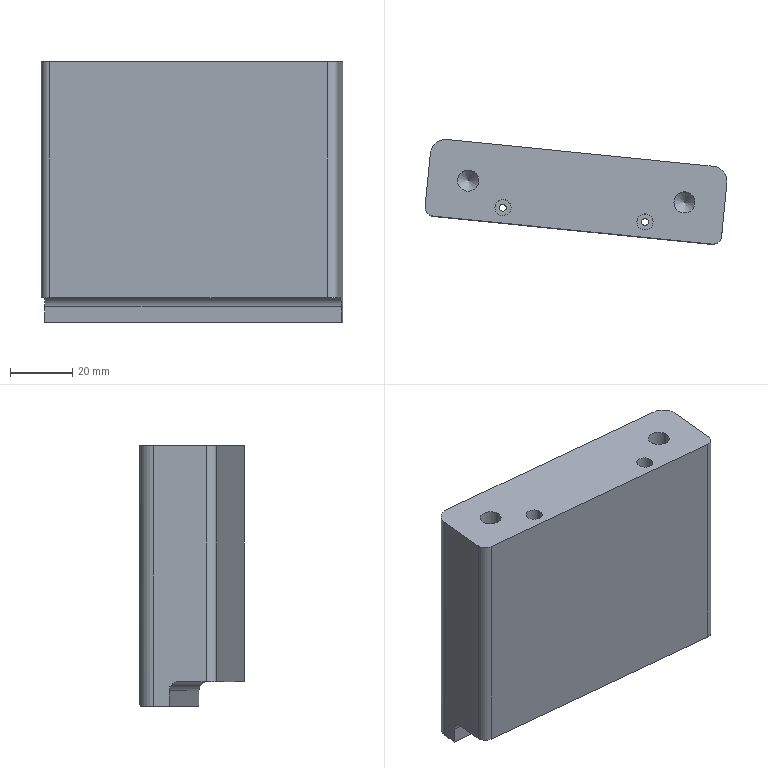Part | NX | features solid 2 | 1 solid | 26 faces | box 97.261 x 33.732 x 84 mm | volume 184630 mm3 | cylinder 13 | plane 10 | cone 3 | commonest cylinder face diameters 5.2 x3 6 x3 2.2 x2 6.8 x2 10 x2 2 x1
STEP:
#1=CARTESIAN_POINT('',(715.348,88.646,-6.));
#2=VERTEX_POINT('',#1);
#3=CARTESIAN_POINT('',(714.248,88.646,-6.));
#4=DIRECTION('',(0.,0.,1.));
#5=DIRECTION('',(1.,0.,0.));
#6=AXIS2_PLACEMENT_3D('',#3,#4,#5);
#7=CIRCLE('',#6,1.1);
#8=EDGE_CURVE('',#2,#2,#7,.F.);
#9=ORIENTED_EDGE('',*,*,#8,.F.);
#10=EDGE_LOOP('',(#9));
#11=FACE_BOUND('',#10,.T.);
#12=CARTESIAN_POINT('',(669.58,93.255,-6.));
#13=VERTEX_POINT('',#12);
#14=CARTESIAN_POINT('',(668.48,93.255,-6.));
#15=DIRECTION('',(0.,0.,1.));
#16=DIRECTION('',(1.,0.,0.));
#17=AXIS2_PLACEMENT_3D('',#14,#15,#16);
#18=CIRCLE('',#17,1.1);
#19=EDGE_CURVE('',#13,#13,#18,.F.);
#20=ORIENTED_EDGE('',*,*,#19,.F.);
#21=EDGE_LOOP('',(#20));
#22=FACE_BOUND('',#21,.T.);
#23=CARTESIAN_POINT('',(644.307,102.725,-6.));
#24=VERTEX_POINT('',#23);
#25=CARTESIAN_POINT('',(690.412,98.082,-6.));
#26=VERTEX_POINT('',#25);
#27=CARTESIAN_POINT('',(753.046,91.775,-6.));
#28=DIRECTION('',(0.995,-0.1002,0.));
#29=VECTOR('',#28,1000.);
#30=LINE('',#27,#29);
#31=EDGE_CURVE('',#24,#26,#30,.T.);
#32=ORIENTED_EDGE('',*,*,#31,.T.);
#33=CARTESIAN_POINT('',(693.718,97.749,-6.));
#34=VERTEX_POINT('',#33);
#35=CARTESIAN_POINT('',(691.865,95.926,-6.));
#36=DIRECTION('',(0.,0.,1.));
#37=DIRECTION('',(1.,0.,0.));
#38=AXIS2_PLACEMENT_3D('',#35,#36,#37);
#39=CIRCLE('',#38,2.6);
#40=EDGE_CURVE('',#26,#34,#39,.T.);
#41=ORIENTED_EDGE('',*,*,#40,.T.);
#42=CARTESIAN_POINT('',(739.824,93.106,-6.));
#43=VERTEX_POINT('',#42);
#44=CARTESIAN_POINT('',(753.046,91.775,-6.));
#45=DIRECTION('',(0.995,-0.1002,0.));
#46=VECTOR('',#45,1000.);
#47=LINE('',#44,#46);
#48=EDGE_CURVE('',#34,#43,#47,.T.);
#49=ORIENTED_EDGE('',*,*,#48,.T.);
#50=CARTESIAN_POINT('',(738.922,84.151,-6.));
#51=VERTEX_POINT('',#50);
#52=CARTESIAN_POINT('',(721.778,-86.088,-6.));
#53=DIRECTION('',(0.1002,0.995,0.));
#54=VECTOR('',#53,1000.);
#55=LINE('',#52,#54);
#56=EDGE_CURVE('',#43,#51,#55,.F.);
#57=ORIENTED_EDGE('',*,*,#56,.T.);
#58=CARTESIAN_POINT('',(735.637,81.467,-6.));
#59=VERTEX_POINT('',#58);
#60=CARTESIAN_POINT('',(735.937,84.452,-6.));
#61=DIRECTION('',(0.,0.,1.));
#62=DIRECTION('',(1.,0.,0.));
#63=AXIS2_PLACEMENT_3D('',#60,#61,#62);
#64=CIRCLE('',#63,3.);
#65=EDGE_CURVE('',#51,#59,#64,.F.);
#66=ORIENTED_EDGE('',*,*,#65,.T.);
#67=CARTESIAN_POINT('',(646.089,90.485,-6.));
#68=VERTEX_POINT('',#67);
#69=CARTESIAN_POINT('',(650.069,90.084,-6.));
#70=DIRECTION('',(-0.995,0.1002,0.));
#71=VECTOR('',#70,1000.);
#72=LINE('',#69,#71);
#73=EDGE_CURVE('',#68,#59,#72,.F.);
#74=ORIENTED_EDGE('',*,*,#73,.F.);
#75=CARTESIAN_POINT('',(643.405,93.77,-6.));
#76=VERTEX_POINT('',#75);
#77=CARTESIAN_POINT('',(646.39,93.47,-6.));
#78=DIRECTION('',(0.,0.,1.));
#79=DIRECTION('',(1.,0.,0.));
#80=AXIS2_PLACEMENT_3D('',#77,#78,#79);
#81=CIRCLE('',#80,3.);
#82=EDGE_CURVE('',#68,#76,#81,.F.);
#83=ORIENTED_EDGE('',*,*,#82,.T.);
#84=CARTESIAN_POINT('',(645.108,110.685,-6.));
#85=DIRECTION('',(0.1002,0.995,0.));
#86=VECTOR('',#85,1000.);
#87=LINE('',#84,#86);
#88=EDGE_CURVE('',#24,#76,#87,.F.);
#89=ORIENTED_EDGE('',*,*,#88,.F.);
#90=EDGE_LOOP('',(#32,#41,#49,#57,#66,#74,#83,#89));
#91=FACE_BOUND('',#90,.T.);
#92=CARTESIAN_POINT('',(735.,-87.419,-6.));
#93=DIRECTION('',(0.,0.,1.));
#94=DIRECTION('',(-0.9997,-0.02352,0.));
#95=AXIS2_PLACEMENT_3D('',#92,#93,#94);
#96=PLANE('',#95);
#97=ADVANCED_FACE('',(#11,#22,#91),#96,.F.);
#98=CARTESIAN_POINT('',(730.339,94.906,70.));
#99=VERTEX_POINT('',#98);
#100=CARTESIAN_POINT('',(726.939,94.906,70.));
#101=DIRECTION('',(0.,0.,-1.));
#102=DIRECTION('',(1.,0.,0.));
#103=AXIS2_PLACEMENT_3D('',#100,#101,#102);
#104=CIRCLE('',#103,3.4);
#105=EDGE_CURVE('',#99,#99,#104,.T.);
#106=ORIENTED_EDGE('',*,*,#105,.T.);
#107=EDGE_LOOP('',(#106));
#108=FACE_BOUND('',#107,.T.);
#109=CARTESIAN_POINT('',(671.08,93.255,70.));
#110=VERTEX_POINT('',#109);
#111=CARTESIAN_POINT('',(668.48,93.255,70.));
#112=DIRECTION('',(0.,0.,1.));
#113=DIRECTION('',(1.,0.,0.));
#114=AXIS2_PLACEMENT_3D('',#111,#112,#113);
#115=CIRCLE('',#114,2.6);
#116=EDGE_CURVE('',#110,#110,#115,.T.);
#117=ORIENTED_EDGE('',*,*,#116,.F.);
#118=EDGE_LOOP('',(#117));
#119=FACE_BOUND('',#118,.T.);
#120=CARTESIAN_POINT('',(716.848,88.646,70.));
#121=VERTEX_POINT('',#120);
#122=CARTESIAN_POINT('',(714.248,88.646,70.));
#123=DIRECTION('',(0.,0.,1.));
#124=DIRECTION('',(1.,0.,0.));
#125=AXIS2_PLACEMENT_3D('',#122,#123,#124);
#126=CIRCLE('',#125,2.6);
#127=EDGE_CURVE('',#121,#121,#126,.T.);
#128=ORIENTED_EDGE('',*,*,#127,.F.);
#129=EDGE_LOOP('',(#128));
#130=FACE_BOUND('',#129,.T.);
#131=CARTESIAN_POINT('',(740.625,101.066,70.));
#132=VERTEX_POINT('',#131);
#133=CARTESIAN_POINT('',(738.922,84.151,70.));
#134=VERTEX_POINT('',#133);
#135=CARTESIAN_POINT('',(740.625,101.066,70.));
#136=DIRECTION('',(-0.1002,-0.995,0.));
#137=VECTOR('',#136,1000.);
#138=LINE('',#135,#137);
#139=EDGE_CURVE('',#132,#134,#138,.T.);
#140=ORIENTED_EDGE('',*,*,#139,.F.);
#141=CARTESIAN_POINT('',(736.152,106.542,70.));
#142=VERTEX_POINT('',#141);
#143=CARTESIAN_POINT('',(735.651,101.567,70.));
#144=DIRECTION('',(0.,0.,1.));
#145=DIRECTION('',(1.,0.,0.));
#146=AXIS2_PLACEMENT_3D('',#143,#144,#145);
#147=CIRCLE('',#146,5.);
#148=EDGE_CURVE('',#132,#142,#147,.T.);
#149=ORIENTED_EDGE('',*,*,#148,.T.);
#150=CARTESIAN_POINT('',(650.584,115.159,70.));
#151=VERTEX_POINT('',#150);
#152=CARTESIAN_POINT('',(652.574,114.958,70.));
#153=DIRECTION('',(-0.995,0.1002,0.));
#154=VECTOR('',#153,1000.);
#155=LINE('',#152,#154);
#156=EDGE_CURVE('',#142,#151,#155,.T.);
#157=ORIENTED_EDGE('',*,*,#156,.T.);
#158=CARTESIAN_POINT('',(645.108,110.685,70.));
#159=VERTEX_POINT('',#158);
#160=CARTESIAN_POINT('',(650.083,110.184,70.));
#161=DIRECTION('',(0.,0.,1.));
#162=DIRECTION('',(1.,0.,0.));
#163=AXIS2_PLACEMENT_3D('',#160,#161,#162);
#164=CIRCLE('',#163,5.);
#165=EDGE_CURVE('',#151,#159,#164,.T.);
#166=ORIENTED_EDGE('',*,*,#165,.T.);
#167=CARTESIAN_POINT('',(643.405,93.77,70.));
#168=VERTEX_POINT('',#167);
#169=CARTESIAN_POINT('',(633.24,-7.174,70.));
#170=DIRECTION('',(-0.1002,-0.995,0.));
#171=VECTOR('',#170,1000.);
#172=LINE('',#169,#171);
#173=EDGE_CURVE('',#159,#168,#172,.T.);
#174=ORIENTED_EDGE('',*,*,#173,.T.);
#175=CARTESIAN_POINT('',(646.089,90.485,70.));
#176=VERTEX_POINT('',#175);
#177=CARTESIAN_POINT('',(646.39,93.47,70.));
#178=DIRECTION('',(0.,0.,1.));
#179=DIRECTION('',(1.,0.,0.));
#180=AXIS2_PLACEMENT_3D('',#177,#178,#179);
#181=CIRCLE('',#180,3.);
#182=EDGE_CURVE('',#168,#176,#181,.T.);
#183=ORIENTED_EDGE('',*,*,#182,.T.);
#184=CARTESIAN_POINT('',(735.637,81.467,70.));
#185=VERTEX_POINT('',#184);
#186=CARTESIAN_POINT('',(650.069,90.084,70.));
#187=DIRECTION('',(-0.995,0.1002,0.));
#188=VECTOR('',#187,1000.);
#189=LINE('',#186,#188);
#190=EDGE_CURVE('',#185,#176,#189,.T.);
#191=ORIENTED_EDGE('',*,*,#190,.F.);
#192=CARTESIAN_POINT('',(735.937,84.452,70.));
#193=DIRECTION('',(0.,0.,1.));
#194=DIRECTION('',(1.,0.,0.));
#195=AXIS2_PLACEMENT_3D('',#192,#193,#194);
#196=CIRCLE('',#195,3.);
#197=EDGE_CURVE('',#185,#134,#196,.T.);
#198=ORIENTED_EDGE('',*,*,#197,.T.);
#199=EDGE_LOOP('',(#140,#149,#157,#166,#174,#183,#191,#198));
#200=FACE_BOUND('',#199,.T.);
#201=CARTESIAN_POINT('',(660.692,101.92,70.));
#202=VERTEX_POINT('',#201);
#203=CARTESIAN_POINT('',(657.292,101.92,70.));
#204=DIRECTION('',(0.,0.,-1.));
#205=DIRECTION('',(1.,0.,0.));
#206=AXIS2_PLACEMENT_3D('',#203,#204,#205);
#207=CIRCLE('',#206,3.4);
#208=EDGE_CURVE('',#202,#202,#207,.T.);
#209=ORIENTED_EDGE('',*,*,#208,.T.);
#210=EDGE_LOOP('',(#209));
#211=FACE_BOUND('',#210,.T.);
#212=CARTESIAN_POINT('',(562.,0.,70.));
#213=DIRECTION('',(0.,0.,1.));
#214=DIRECTION('',(1.,0.,0.));
#215=AXIS2_PLACEMENT_3D('',#212,#213,#214);
#216=PLANE('',#215);
#217=ADVANCED_FACE('',(#108,#119,#130,#200,#211),#216,.T.);
#218=ORIENTED_EDGE('',*,*,#173,.F.);
#219=CARTESIAN_POINT('',(645.108,110.685,-14.));
#220=VERTEX_POINT('',#219);
#221=CARTESIAN_POINT('',(645.108,110.685,-14.));
#222=DIRECTION('',(0.,0.,-1.));
#223=VECTOR('',#222,1000.);
#224=LINE('',#221,#223);
#225=EDGE_CURVE('',#159,#220,#224,.T.);
#226=ORIENTED_EDGE('',*,*,#225,.T.);
#227=CARTESIAN_POINT('',(644.607,105.71,-14.));
#228=VERTEX_POINT('',#227);
#229=CARTESIAN_POINT('',(645.108,110.685,-14.));
#230=DIRECTION('',(-0.1002,-0.995,0.));
#231=VECTOR('',#230,1000.);
#232=LINE('',#229,#231);
#233=EDGE_CURVE('',#220,#228,#232,.T.);
#234=ORIENTED_EDGE('',*,*,#233,.T.);
#235=CARTESIAN_POINT('',(644.607,105.71,-9.));
#236=VERTEX_POINT('',#235);
#237=CARTESIAN_POINT('',(644.607,105.71,-41.49));
#238=DIRECTION('',(0.,0.,-1.));
#239=VECTOR('',#238,1000.);
#240=LINE('',#237,#239);
#241=EDGE_CURVE('',#228,#236,#240,.F.);
#242=ORIENTED_EDGE('',*,*,#241,.T.);
#243=CARTESIAN_POINT('',(644.307,102.725,-9.));
#244=DIRECTION('',(-0.995,0.1002,0.));
#245=DIRECTION('',(-0.1002,-0.995,0.));
#246=AXIS2_PLACEMENT_3D('',#243,#244,#245);
#247=CIRCLE('',#246,3.);
#248=EDGE_CURVE('',#236,#24,#247,.F.);
#249=ORIENTED_EDGE('',*,*,#248,.T.);
#250=ORIENTED_EDGE('',*,*,#88,.T.);
#251=CARTESIAN_POINT('',(643.405,93.77,-41.49));
#252=DIRECTION('',(0.,0.,-1.));
#253=VECTOR('',#252,1000.);
#254=LINE('',#251,#253);
#255=EDGE_CURVE('',#76,#168,#254,.F.);
#256=ORIENTED_EDGE('',*,*,#255,.T.);
#257=EDGE_LOOP('',(#218,#226,#234,#242,#249,#250,#256));
#258=FACE_BOUND('',#257,.T.);
#259=CARTESIAN_POINT('',(645.108,110.685,-41.49));
#260=DIRECTION('',(-0.995,0.1002,0.));
#261=DIRECTION('',(-0.1002,-0.995,0.));
#262=AXIS2_PLACEMENT_3D('',#259,#260,#261);
#263=PLANE('',#262);
#264=ADVANCED_FACE('',(#258),#263,.T.);
#265=CARTESIAN_POINT('',(740.625,101.066,-14.));
#266=VERTEX_POINT('',#265);
#267=CARTESIAN_POINT('',(740.124,96.091,-14.));
#268=VERTEX_POINT('',#267);
#269=CARTESIAN_POINT('',(712.51,-178.12,-14.));
#270=DIRECTION('',(-0.1002,-0.995,0.));
#271=VECTOR('',#270,1000.);
#272=LINE('',#269,#271);
#273=EDGE_CURVE('',#266,#268,#272,.T.);
#274=ORIENTED_EDGE('',*,*,#273,.F.);
#275=CARTESIAN_POINT('',(740.625,101.066,50.));
#276=DIRECTION('',(0.,0.,1.));
#277=VECTOR('',#276,1000.);
#278=LINE('',#275,#277);
#279=EDGE_CURVE('',#266,#132,#278,.T.);
#280=ORIENTED_EDGE('',*,*,#279,.T.);
#281=ORIENTED_EDGE('',*,*,#139,.T.);
#282=CARTESIAN_POINT('',(738.922,84.151,-41.49));
#283=DIRECTION('',(0.,0.,1.));
#284=VECTOR('',#283,1000.);
#285=LINE('',#282,#284);
#286=EDGE_CURVE('',#134,#51,#285,.F.);
#287=ORIENTED_EDGE('',*,*,#286,.T.);
#288=ORIENTED_EDGE('',*,*,#56,.F.);
#289=CARTESIAN_POINT('',(740.124,96.091,-9.));
#290=VERTEX_POINT('',#289);
#291=CARTESIAN_POINT('',(739.824,93.106,-9.));
#292=DIRECTION('',(0.995,-0.1002,0.));
#293=DIRECTION('',(0.1002,0.995,0.));
#294=AXIS2_PLACEMENT_3D('',#291,#292,#293);
#295=CIRCLE('',#294,3.);
#296=EDGE_CURVE('',#43,#290,#295,.F.);
#297=ORIENTED_EDGE('',*,*,#296,.T.);
#298=CARTESIAN_POINT('',(740.124,96.091,-41.49));
#299=DIRECTION('',(0.,0.,1.));
#300=VECTOR('',#299,1000.);
#301=LINE('',#298,#300);
#302=EDGE_CURVE('',#268,#290,#301,.T.);
#303=ORIENTED_EDGE('',*,*,#302,.F.);
#304=EDGE_LOOP('',(#274,#280,#281,#287,#288,#297,#303));
#305=FACE_BOUND('',#304,.T.);
#306=CARTESIAN_POINT('',(740.625,101.066,-41.49));
#307=DIRECTION('',(0.995,-0.1002,0.));
#308=DIRECTION('',(0.1002,0.995,0.));
#309=AXIS2_PLACEMENT_3D('',#306,#307,#308);
#310=PLANE('',#309);
#311=ADVANCED_FACE('',(#305),#310,.T.);
#312=ORIENTED_EDGE('',*,*,#73,.T.);
#313=CARTESIAN_POINT('',(735.637,81.467,-41.49));
#314=DIRECTION('',(0.,0.,1.));
#315=VECTOR('',#314,1000.);
#316=LINE('',#313,#315);
#317=EDGE_CURVE('',#59,#185,#316,.T.);
#318=ORIENTED_EDGE('',*,*,#317,.T.);
#319=ORIENTED_EDGE('',*,*,#190,.T.);
#320=CARTESIAN_POINT('',(646.089,90.485,-41.49));
#321=DIRECTION('',(0.,0.,-1.));
#322=VECTOR('',#321,1000.);
#323=LINE('',#320,#322);
#324=EDGE_CURVE('',#176,#68,#323,.T.);
#325=ORIENTED_EDGE('',*,*,#324,.T.);
#326=EDGE_LOOP('',(#312,#318,#319,#325));
#327=FACE_BOUND('',#326,.T.);
#328=CARTESIAN_POINT('',(650.069,90.084,-41.49));
#329=DIRECTION('',(-0.1002,-0.995,0.));
#330=DIRECTION('',(0.995,-0.1002,0.));
#331=AXIS2_PLACEMENT_3D('',#328,#329,#330);
#332=PLANE('',#331);
#333=ADVANCED_FACE('',(#327),#332,.T.);
#334=ORIENTED_EDGE('',*,*,#65,.F.);
#335=ORIENTED_EDGE('',*,*,#286,.F.);
#336=ORIENTED_EDGE('',*,*,#197,.F.);
#337=ORIENTED_EDGE('',*,*,#317,.F.);
#338=EDGE_LOOP('',(#334,#335,#336,#337));
#339=FACE_BOUND('',#338,.T.);
#340=CARTESIAN_POINT('',(735.937,84.452,-41.49));
#341=DIRECTION('',(0.,0.,1.));
#342=DIRECTION('',(1.,0.,0.));
#343=AXIS2_PLACEMENT_3D('',#340,#341,#342);
#344=CYLINDRICAL_SURFACE('',#343,3.);
#345=ADVANCED_FACE('',(#339),#344,.T.);
#346=ORIENTED_EDGE('',*,*,#182,.F.);
#347=ORIENTED_EDGE('',*,*,#255,.F.);
#348=ORIENTED_EDGE('',*,*,#82,.F.);
#349=ORIENTED_EDGE('',*,*,#324,.F.);
#350=EDGE_LOOP('',(#346,#347,#348,#349));
#351=FACE_BOUND('',#350,.T.);
#352=CARTESIAN_POINT('',(646.39,93.47,-41.49));
#353=DIRECTION('',(0.,0.,-1.));
#354=DIRECTION('',(-1.,0.,0.));
#355=AXIS2_PLACEMENT_3D('',#352,#353,#354);
#356=CYLINDRICAL_SURFACE('',#355,3.);
#357=ADVANCED_FACE('',(#351),#356,.T.);
#358=CARTESIAN_POINT('',(736.152,106.542,-13.));
#359=VERTEX_POINT('',#358);
#360=CARTESIAN_POINT('',(736.152,106.542,-14.));
#361=DIRECTION('',(0.,0.,1.));
#362=VECTOR('',#361,1000.);
#363=LINE('',#360,#362);
#364=EDGE_CURVE('',#142,#359,#363,.F.);
#365=ORIENTED_EDGE('',*,*,#364,.T.);
#366=CARTESIAN_POINT('',(650.584,115.159,-13.));
#367=VERTEX_POINT('',#366);
#368=CARTESIAN_POINT('',(650.584,115.159,-13.));
#369=DIRECTION('',(0.995,-0.1002,0.));
#370=VECTOR('',#369,1000.);
#371=LINE('',#368,#370);
#372=EDGE_CURVE('',#359,#367,#371,.F.);
#373=ORIENTED_EDGE('',*,*,#372,.T.);
#374=CARTESIAN_POINT('',(650.584,115.159,50.));
#375=DIRECTION('',(0.,0.,-1.));
#376=VECTOR('',#375,1000.);
#377=LINE('',#374,#376);
#378=EDGE_CURVE('',#367,#151,#377,.F.);
#379=ORIENTED_EDGE('',*,*,#378,.T.);
#380=ORIENTED_EDGE('',*,*,#156,.F.);
#381=EDGE_LOOP('',(#365,#373,#379,#380));
#382=FACE_BOUND('',#381,.T.);
#383=CARTESIAN_POINT('',(652.574,114.958,-41.49));
#384=DIRECTION('',(-0.1002,-0.995,0.));
#385=DIRECTION('',(0.995,-0.1002,0.));
#386=AXIS2_PLACEMENT_3D('',#383,#384,#385);
#387=PLANE('',#386);
#388=ADVANCED_FACE('',(#382),#387,.F.);
#389=CARTESIAN_POINT('',(647.499,114.464,-14.));
#390=VERTEX_POINT('',#389);
#391=CARTESIAN_POINT('',(650.083,110.184,-14.));
#392=DIRECTION('',(0.,0.,-1.));
#393=DIRECTION('',(-1.,0.,0.));
#394=AXIS2_PLACEMENT_3D('',#391,#392,#393);
#395=CIRCLE('',#394,5.);
#396=EDGE_CURVE('',#220,#390,#395,.T.);
#397=ORIENTED_EDGE('',*,*,#396,.T.);
#398=CARTESIAN_POINT('',(739.036,105.246,-14.));
#399=VERTEX_POINT('',#398);
#400=CARTESIAN_POINT('',(736.051,105.547,-14.));
#401=DIRECTION('',(0.995,-0.1002,0.));
#402=VECTOR('',#401,1000.);
#403=LINE('',#400,#402);
#404=EDGE_CURVE('',#390,#399,#403,.T.);
#405=ORIENTED_EDGE('',*,*,#404,.T.);
#406=CARTESIAN_POINT('',(735.651,101.567,-14.));
#407=DIRECTION('',(0.,0.,-1.));
#408=DIRECTION('',(-1.,0.,0.));
#409=AXIS2_PLACEMENT_3D('',#406,#407,#408);
#410=CIRCLE('',#409,5.);
#411=EDGE_CURVE('',#399,#266,#410,.T.);
#412=ORIENTED_EDGE('',*,*,#411,.T.);
#413=ORIENTED_EDGE('',*,*,#273,.T.);
#414=CARTESIAN_POINT('',(692.366,100.901,-14.));
#415=DIRECTION('',(-0.995,0.1002,0.));
#416=VECTOR('',#415,1000.);
#417=LINE('',#414,#416);
#418=EDGE_CURVE('',#268,#228,#417,.T.);
#419=ORIENTED_EDGE('',*,*,#418,.T.);
#420=ORIENTED_EDGE('',*,*,#233,.F.);
#421=EDGE_LOOP('',(#397,#405,#412,#413,#419,#420));
#422=FACE_BOUND('',#421,.T.);
#423=CARTESIAN_POINT('',(16.212,-108.,-14.));
#424=DIRECTION('',(0.,0.,-1.));
#425=DIRECTION('',(-1.,0.,0.));
#426=AXIS2_PLACEMENT_3D('',#423,#424,#425);
#427=PLANE('',#426);
#428=ADVANCED_FACE('',(#422),#427,.T.);
#429=ORIENTED_EDGE('',*,*,#302,.T.);
#430=CARTESIAN_POINT('',(692.366,100.901,-9.));
#431=DIRECTION('',(-0.995,0.1002,0.));
#432=VECTOR('',#431,1000.);
#433=LINE('',#430,#432);
#434=EDGE_CURVE('',#290,#236,#433,.T.);
#435=ORIENTED_EDGE('',*,*,#434,.T.);
#436=ORIENTED_EDGE('',*,*,#241,.F.);
#437=ORIENTED_EDGE('',*,*,#418,.F.);
#438=EDGE_LOOP('',(#429,#435,#436,#437));
#439=FACE_BOUND('',#438,.T.);
#440=CARTESIAN_POINT('',(692.366,100.901,18.));
#441=DIRECTION('',(0.1002,0.995,0.));
#442=DIRECTION('',(-0.995,0.1002,0.));
#443=AXIS2_PLACEMENT_3D('',#440,#441,#442);
#444=PLANE('',#443);
#445=ADVANCED_FACE('',(#439),#444,.F.);
#446=ORIENTED_EDGE('',*,*,#411,.F.);
#447=CARTESIAN_POINT('',(739.036,105.246,-14.));
#448=CARTESIAN_POINT('',(738.194,106.021,-14.));
#449=CARTESIAN_POINT('',(737.177,106.438,-13.461));
#450=CARTESIAN_POINT('',(736.152,106.542,-13.));
#451=B_SPLINE_CURVE_WITH_KNOTS('',3,(#447,#448,#449,#450),.UNSPECIFIED.,.F.,.F.,(4,4),(0.,0.003386),.UNSPECIFIED.);
#452=EDGE_CURVE('',#399,#359,#451,.T.);
#453=ORIENTED_EDGE('',*,*,#452,.T.);
#454=ORIENTED_EDGE('',*,*,#364,.F.);
#455=ORIENTED_EDGE('',*,*,#148,.F.);
#456=ORIENTED_EDGE('',*,*,#279,.F.);
#457=EDGE_LOOP('',(#446,#453,#454,#455,#456));
#458=FACE_BOUND('',#457,.T.);
#459=CARTESIAN_POINT('',(735.651,101.567,-41.49));
#460=DIRECTION('',(0.,0.,-1.));
#461=DIRECTION('',(-1.,0.,0.));
#462=AXIS2_PLACEMENT_3D('',#459,#460,#461);
#463=CYLINDRICAL_SURFACE('',#462,5.);
#464=ADVANCED_FACE('',(#458),#463,.T.);
#465=ORIENTED_EDGE('',*,*,#378,.F.);
#466=CARTESIAN_POINT('',(647.499,114.464,-14.));
#467=CARTESIAN_POINT('',(648.478,115.056,-14.));
#468=CARTESIAN_POINT('',(649.559,115.262,-13.461));
#469=CARTESIAN_POINT('',(650.584,115.159,-13.));
#470=B_SPLINE_CURVE_WITH_KNOTS('',3,(#466,#467,#468,#469),.UNSPECIFIED.,.F.,.F.,(4,4),(0.,0.003386),.UNSPECIFIED.);
#471=EDGE_CURVE('',#367,#390,#470,.F.);
#472=ORIENTED_EDGE('',*,*,#471,.T.);
#473=ORIENTED_EDGE('',*,*,#396,.F.);
#474=ORIENTED_EDGE('',*,*,#225,.F.);
#475=ORIENTED_EDGE('',*,*,#165,.F.);
#476=EDGE_LOOP('',(#465,#472,#473,#474,#475));
#477=FACE_BOUND('',#476,.T.);
#478=CARTESIAN_POINT('',(650.083,110.184,-41.49));
#479=DIRECTION('',(0.,0.,1.));
#480=DIRECTION('',(1.,0.,0.));
#481=AXIS2_PLACEMENT_3D('',#478,#479,#480);
#482=CYLINDRICAL_SURFACE('',#481,5.);
#483=ADVANCED_FACE('',(#477),#482,.T.);
#484=CARTESIAN_POINT('',(690.412,98.082,-6.));
#485=CARTESIAN_POINT('',(690.916,98.421,-6.));
#486=CARTESIAN_POINT('',(692.146,98.724,-6.121));
#487=CARTESIAN_POINT('',(693.293,98.182,-6.));
#488=CARTESIAN_POINT('',(693.718,97.749,-6.));
#489=B_SPLINE_CURVE_WITH_KNOTS('',3,(#484,#485,#486,#487,#488),.UNSPECIFIED.,.F.,.F.,(4,1,4),(0.,0.001794,0.003588),.UNSPECIFIED.);
#490=EDGE_CURVE('',#26,#34,#489,.T.);
#491=ORIENTED_EDGE('',*,*,#490,.F.);
#492=ORIENTED_EDGE('',*,*,#31,.F.);
#493=ORIENTED_EDGE('',*,*,#248,.F.);
#494=ORIENTED_EDGE('',*,*,#434,.F.);
#495=ORIENTED_EDGE('',*,*,#296,.F.);
#496=ORIENTED_EDGE('',*,*,#48,.F.);
#497=EDGE_LOOP('',(#491,#492,#493,#494,#495,#496));
#498=FACE_BOUND('',#497,.T.);
#499=CARTESIAN_POINT('',(753.046,91.775,-9.));
#500=DIRECTION('',(-0.995,0.1002,0.));
#501=DIRECTION('',(-0.1002,-0.995,0.));
#502=AXIS2_PLACEMENT_3D('',#499,#500,#501);
#503=CYLINDRICAL_SURFACE('',#502,3.);
#504=ADVANCED_FACE('',(#498),#503,.F.);
#505=ORIENTED_EDGE('',*,*,#8,.T.);
#506=EDGE_LOOP('',(#505));
#507=FACE_BOUND('',#506,.T.);
#508=CARTESIAN_POINT('',(713.148,88.646,29.));
#509=VERTEX_POINT('',#508);
#510=CARTESIAN_POINT('',(714.248,88.646,29.));
#511=DIRECTION('',(0.,0.,-1.));
#512=DIRECTION('',(-1.,0.,0.));
#513=AXIS2_PLACEMENT_3D('',#510,#511,#512);
#514=CIRCLE('',#513,1.1);
#515=EDGE_CURVE('',#509,#509,#514,.T.);
#516=ORIENTED_EDGE('',*,*,#515,.F.);
#517=EDGE_LOOP('',(#516));
#518=FACE_BOUND('',#517,.T.);
#519=CARTESIAN_POINT('',(714.248,88.646,32.));
#520=DIRECTION('',(0.,0.,-1.));
#521=DIRECTION('',(1.,0.,0.));
#522=AXIS2_PLACEMENT_3D('',#519,#520,#521);
#523=CYLINDRICAL_SURFACE('',#522,1.1);
#524=ADVANCED_FACE('',(#507,#518),#523,.F.);
#525=ORIENTED_EDGE('',*,*,#515,.T.);
#526=EDGE_LOOP('',(#525));
#527=FACE_BOUND('',#526,.T.);
#528=CARTESIAN_POINT('',(716.848,88.646,29.));
#529=VERTEX_POINT('',#528);
#530=CARTESIAN_POINT('',(714.248,88.646,29.));
#531=DIRECTION('',(0.,0.,1.));
#532=DIRECTION('',(1.,0.,0.));
#533=AXIS2_PLACEMENT_3D('',#530,#531,#532);
#534=CIRCLE('',#533,2.6);
#535=EDGE_CURVE('',#529,#529,#534,.F.);
#536=ORIENTED_EDGE('',*,*,#535,.F.);
#537=EDGE_LOOP('',(#536));
#538=FACE_BOUND('',#537,.T.);
#539=CARTESIAN_POINT('',(714.248,88.646,29.));
#540=DIRECTION('',(0.,0.,-1.));
#541=DIRECTION('',(-1.,0.,0.));
#542=AXIS2_PLACEMENT_3D('',#539,#540,#541);
#543=PLANE('',#542);
#544=ADVANCED_FACE('',(#527,#538),#543,.F.);
#545=ORIENTED_EDGE('',*,*,#127,.T.);
#546=EDGE_LOOP('',(#545));
#547=FACE_BOUND('',#546,.T.);
#548=ORIENTED_EDGE('',*,*,#535,.T.);
#549=EDGE_LOOP('',(#548));
#550=FACE_BOUND('',#549,.T.);
#551=CARTESIAN_POINT('',(714.248,88.646,29.));
#552=DIRECTION('',(0.,0.,1.));
#553=DIRECTION('',(1.,0.,0.));
#554=AXIS2_PLACEMENT_3D('',#551,#552,#553);
#555=CYLINDRICAL_SURFACE('',#554,2.6);
#556=ADVANCED_FACE('',(#547,#550),#555,.F.);
#557=ORIENTED_EDGE('',*,*,#19,.T.);
#558=EDGE_LOOP('',(#557));
#559=FACE_BOUND('',#558,.T.);
#560=CARTESIAN_POINT('',(669.558,93.036,29.));
#561=VERTEX_POINT('',#560);
#562=CARTESIAN_POINT('',(668.48,93.255,29.));
#563=DIRECTION('',(0.,0.,1.));
#564=DIRECTION('',(0.9799,-0.1994,0.));
#565=AXIS2_PLACEMENT_3D('',#562,#563,#564);
#566=CIRCLE('',#565,1.1);
#567=EDGE_CURVE('',#561,#561,#566,.T.);
#568=ORIENTED_EDGE('',*,*,#567,.T.);
#569=EDGE_LOOP('',(#568));
#570=FACE_BOUND('',#569,.T.);
#571=CARTESIAN_POINT('',(668.48,93.255,32.));
#572=DIRECTION('',(0.,0.,-1.));
#573=DIRECTION('',(-0.9799,0.1994,0.));
#574=AXIS2_PLACEMENT_3D('',#571,#572,#573);
#575=CYLINDRICAL_SURFACE('',#574,1.1);
#576=ADVANCED_FACE('',(#559,#570),#575,.F.);
#577=ORIENTED_EDGE('',*,*,#567,.F.);
#578=EDGE_LOOP('',(#577));
#579=FACE_BOUND('',#578,.T.);
#580=CARTESIAN_POINT('',(665.932,93.774,29.));
#581=VERTEX_POINT('',#580);
#582=CARTESIAN_POINT('',(668.48,93.255,29.));
#583=DIRECTION('',(0.,0.,-1.));
#584=DIRECTION('',(-0.9799,0.1994,0.));
#585=AXIS2_PLACEMENT_3D('',#582,#583,#584);
#586=CIRCLE('',#585,2.6);
#587=EDGE_CURVE('',#581,#581,#586,.F.);
#588=ORIENTED_EDGE('',*,*,#587,.T.);
#589=EDGE_LOOP('',(#588));
#590=FACE_BOUND('',#589,.T.);
#591=CARTESIAN_POINT('',(668.48,93.255,29.));
#592=DIRECTION('',(0.,0.,-1.));
#593=DIRECTION('',(0.9799,-0.1994,0.));
#594=AXIS2_PLACEMENT_3D('',#591,#592,#593);
#595=PLANE('',#594);
#596=ADVANCED_FACE('',(#579,#590),#595,.F.);
#597=ORIENTED_EDGE('',*,*,#116,.T.);
#598=EDGE_LOOP('',(#597));
#599=FACE_BOUND('',#598,.T.);
#600=ORIENTED_EDGE('',*,*,#587,.F.);
#601=EDGE_LOOP('',(#600));
#602=FACE_BOUND('',#601,.T.);
#603=CARTESIAN_POINT('',(668.48,93.255,29.));
#604=DIRECTION('',(0.,0.,1.));
#605=DIRECTION('',(-0.9799,0.1994,0.));
#606=AXIS2_PLACEMENT_3D('',#603,#604,#605);
#607=CYLINDRICAL_SURFACE('',#606,2.6);
#608=ADVANCED_FACE('',(#599,#602),#607,.F.);
#609=ORIENTED_EDGE('',*,*,#471,.F.);
#610=ORIENTED_EDGE('',*,*,#372,.F.);
#611=ORIENTED_EDGE('',*,*,#452,.F.);
#612=ORIENTED_EDGE('',*,*,#404,.F.);
#613=EDGE_LOOP('',(#609,#610,#611,#612));
#614=FACE_BOUND('',#613,.T.);
#615=CARTESIAN_POINT('',(44.729,175.166,-13.));
#616=DIRECTION('',(-0.995,0.1002,0.));
#617=DIRECTION('',(-0.1002,-0.995,0.));
#618=AXIS2_PLACEMENT_3D('',#615,#616,#617);
#619=CYLINDRICAL_SURFACE('',#618,1.);
#620=ADVANCED_FACE('',(#614),#619,.T.);
#621=CARTESIAN_POINT('',(723.539,94.906,44.4));
#622=VERTEX_POINT('',#621);
#623=CARTESIAN_POINT('',(726.939,94.906,44.4));
#624=DIRECTION('',(0.,0.,-1.));
#625=DIRECTION('',(-1.,0.,0.));
#626=AXIS2_PLACEMENT_3D('',#623,#624,#625);
#627=CIRCLE('',#626,3.4);
#628=EDGE_CURVE('',#622,#622,#627,.T.);
#629=ORIENTED_EDGE('',*,*,#628,.T.);
#630=EDGE_LOOP('',(#629));
#631=FACE_BOUND('',#630,.T.);
#632=ORIENTED_EDGE('',*,*,#105,.F.);
#633=EDGE_LOOP('',(#632));
#634=FACE_BOUND('',#633,.T.);
#635=CARTESIAN_POINT('',(726.939,94.906,70.));
#636=DIRECTION('',(0.,0.,-1.));
#637=DIRECTION('',(1.,0.,0.));
#638=AXIS2_PLACEMENT_3D('',#635,#636,#637);
#639=CYLINDRICAL_SURFACE('',#638,3.4);
#640=ADVANCED_FACE('',(#631,#634),#639,.F.);
#641=CARTESIAN_POINT('',(726.939,94.906,41.));
#642=VERTEX_POINT('',#641);
#643=VERTEX_LOOP('',#642);
#644=FACE_BOUND('',#643,.T.);
#645=ORIENTED_EDGE('',*,*,#628,.F.);
#646=EDGE_LOOP('',(#645));
#647=FACE_BOUND('',#646,.T.);
#648=CARTESIAN_POINT('',(726.939,94.906,44.4));
#649=DIRECTION('',(0.,0.,1.));
#650=DIRECTION('',(1.,0.,0.));
#651=AXIS2_PLACEMENT_3D('',#648,#649,#650);
#652=CONICAL_SURFACE('',#651,3.4,0.7854);
#653=ADVANCED_FACE('',(#644,#647),#652,.F.);
#654=CARTESIAN_POINT('',(653.892,101.92,44.4));
#655=VERTEX_POINT('',#654);
#656=CARTESIAN_POINT('',(657.292,101.92,44.4));
#657=DIRECTION('',(0.,0.,-1.));
#658=DIRECTION('',(-1.,0.,0.));
#659=AXIS2_PLACEMENT_3D('',#656,#657,#658);
#660=CIRCLE('',#659,3.4);
#661=EDGE_CURVE('',#655,#655,#660,.T.);
#662=ORIENTED_EDGE('',*,*,#661,.T.);
#663=EDGE_LOOP('',(#662));
#664=FACE_BOUND('',#663,.T.);
#665=ORIENTED_EDGE('',*,*,#208,.F.);
#666=EDGE_LOOP('',(#665));
#667=FACE_BOUND('',#666,.T.);
#668=CARTESIAN_POINT('',(657.292,101.92,70.));
#669=DIRECTION('',(0.,0.,-1.));
#670=DIRECTION('',(1.,0.,0.));
#671=AXIS2_PLACEMENT_3D('',#668,#669,#670);
#672=CYLINDRICAL_SURFACE('',#671,3.4);
#673=ADVANCED_FACE('',(#664,#667),#672,.F.);
#674=CARTESIAN_POINT('',(657.292,101.92,41.));
#675=VERTEX_POINT('',#674);
#676=VERTEX_LOOP('',#675);
#677=FACE_BOUND('',#676,.T.);
#678=ORIENTED_EDGE('',*,*,#661,.F.);
#679=EDGE_LOOP('',(#678));
#680=FACE_BOUND('',#679,.T.);
#681=CARTESIAN_POINT('',(657.292,101.92,44.4));
#682=DIRECTION('',(0.,0.,1.));
#683=DIRECTION('',(1.,0.,0.));
#684=AXIS2_PLACEMENT_3D('',#681,#682,#683);
#685=CONICAL_SURFACE('',#684,3.4,0.7854);
#686=ADVANCED_FACE('',(#677,#680),#685,.F.);
#687=CARTESIAN_POINT('',(689.265,95.926,15.4));
#688=VERTEX_POINT('',#687);
#689=CARTESIAN_POINT('',(691.865,95.926,15.4));
#690=DIRECTION('',(0.,0.,-1.));
#691=DIRECTION('',(-1.,0.,0.));
#692=AXIS2_PLACEMENT_3D('',#689,#690,#691);
#693=CIRCLE('',#692,2.6);
#694=EDGE_CURVE('',#688,#688,#693,.F.);
#695=ORIENTED_EDGE('',*,*,#694,.T.);
#696=EDGE_LOOP('',(#695));
#697=FACE_BOUND('',#696,.T.);
#698=ORIENTED_EDGE('',*,*,#490,.T.);
#699=ORIENTED_EDGE('',*,*,#40,.F.);
#700=EDGE_LOOP('',(#698,#699));
#701=FACE_BOUND('',#700,.T.);
#702=CARTESIAN_POINT('',(691.865,95.926,-6.));
#703=DIRECTION('',(0.,0.,1.));
#704=DIRECTION('',(1.,0.,0.));
#705=AXIS2_PLACEMENT_3D('',#702,#703,#704);
#706=CYLINDRICAL_SURFACE('',#705,2.6);
#707=ADVANCED_FACE('',(#697,#701),#706,.F.);
#708=CARTESIAN_POINT('',(691.865,95.926,18.));
#709=VERTEX_POINT('',#708);
#710=VERTEX_LOOP('',#709);
#711=FACE_BOUND('',#710,.T.);
#712=ORIENTED_EDGE('',*,*,#694,.F.);
#713=EDGE_LOOP('',(#712));
#714=FACE_BOUND('',#713,.T.);
#715=CARTESIAN_POINT('',(691.865,95.926,15.4));
#716=DIRECTION('',(0.,0.,-1.));
#717=DIRECTION('',(-1.,0.,0.));
#718=AXIS2_PLACEMENT_3D('',#715,#716,#717);
#719=CONICAL_SURFACE('',#718,2.599,0.7854);
#720=ADVANCED_FACE('',(#711,#714),#719,.F.);
#721=CLOSED_SHELL('',(#97,#217,#264,#311,#333,#345,#357,#388,#428,#445,#464,#483,#504,#524,#544,#556,#576,#596,#608,#620,#640,#653,#673,#686,#707,#720));
#722=MANIFOLD_SOLID_BREP('',#721);
#723=(LENGTH_UNIT()NAMED_UNIT(*)SI_UNIT(.MILLI.,.METRE.));
#724=UNCERTAINTY_MEASURE_WITH_UNIT(LENGTH_MEASURE(0.0508),#723,'','');
#725=(NAMED_UNIT(*)PLANE_ANGLE_UNIT()SI_UNIT($,.RADIAN.));
#726=(NAMED_UNIT(*)SI_UNIT($,.STERADIAN.)SOLID_ANGLE_UNIT());
#727=(GEOMETRIC_REPRESENTATION_CONTEXT(3)GLOBAL_UNCERTAINTY_ASSIGNED_CONTEXT((#724))GLOBAL_UNIT_ASSIGNED_CONTEXT((#723,#725,#726))REPRESENTATION_CONTEXT('',''));
#728=ADVANCED_BREP_SHAPE_REPRESENTATION('',(#722),#727);